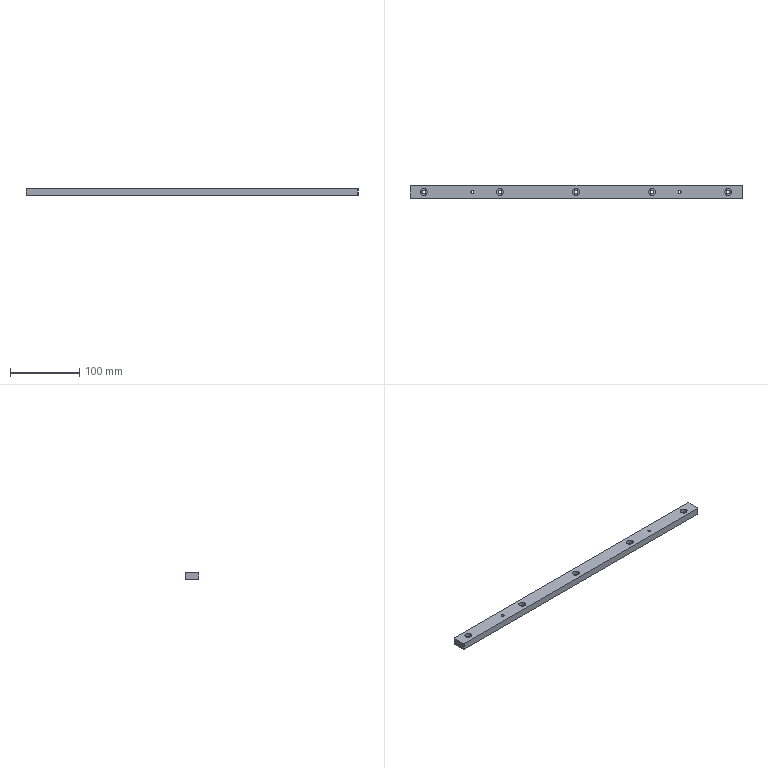Part | SolidWorks | features HoleWzd 2, Chamfer 1, Extrusion 1 | 1 solid | 39 faces | box 480 x 20 x 10 mm | volume 92979 mm3 | cylinder 24 | plane 15 | commonest cylinder face diameters 5.5 x10 10 x10 4 x4
STEP:
#1=CARTESIAN_POINT('',(-152.,0.,0.));
#2=VERTEX_POINT('',#1);
#3=CARTESIAN_POINT('',(-148.,0.,0.));
#4=VERTEX_POINT('',#3);
#5=CARTESIAN_POINT('',(-150.,0.,0.));
#6=DIRECTION('',(0.,0.,1.));
#7=DIRECTION('',(1.,0.,0.));
#8=AXIS2_PLACEMENT_3D('',#5,#6,#7);
#9=CIRCLE('',#8,2.);
#10=EDGE_CURVE('',#2,#4,#9,.T.);
#11=ORIENTED_EDGE('',*,*,#10,.F.);
#12=CARTESIAN_POINT('',(-152.,0.,10.));
#13=VERTEX_POINT('',#12);
#14=CARTESIAN_POINT('',(-152.,0.,10.));
#15=DIRECTION('',(0.,0.,1.));
#16=VECTOR('',#15,1000.);
#17=LINE('',#14,#16);
#18=EDGE_CURVE('',#2,#13,#17,.T.);
#19=ORIENTED_EDGE('',*,*,#18,.T.);
#20=CARTESIAN_POINT('',(-148.,0.,10.));
#21=VERTEX_POINT('',#20);
#22=CARTESIAN_POINT('',(-150.,0.,10.));
#23=DIRECTION('',(0.,0.,1.));
#24=DIRECTION('',(1.,0.,0.));
#25=AXIS2_PLACEMENT_3D('',#22,#23,#24);
#26=CIRCLE('',#25,2.);
#27=EDGE_CURVE('',#13,#21,#26,.T.);
#28=ORIENTED_EDGE('',*,*,#27,.T.);
#29=CARTESIAN_POINT('',(-148.,0.,10.));
#30=DIRECTION('',(0.,0.,1.));
#31=VECTOR('',#30,1000.);
#32=LINE('',#29,#31);
#33=EDGE_CURVE('',#4,#21,#32,.T.);
#34=ORIENTED_EDGE('',*,*,#33,.F.);
#35=EDGE_LOOP('',(#11,#19,#28,#34));
#36=FACE_OUTER_BOUND('',#35,.T.);
#37=CARTESIAN_POINT('',(-150.,0.,10.));
#38=DIRECTION('',(0.,0.,1.));
#39=DIRECTION('',(1.,0.,0.));
#40=AXIS2_PLACEMENT_3D('',#37,#38,#39);
#41=CYLINDRICAL_SURFACE('',#40,2.);
#42=ADVANCED_FACE('',(#36),#41,.F.);
#43=CARTESIAN_POINT('',(148.,0.,0.));
#44=VERTEX_POINT('',#43);
#45=CARTESIAN_POINT('',(152.,0.,0.));
#46=VERTEX_POINT('',#45);
#47=CARTESIAN_POINT('',(150.,0.,0.));
#48=DIRECTION('',(0.,0.,1.));
#49=DIRECTION('',(1.,0.,0.));
#50=AXIS2_PLACEMENT_3D('',#47,#48,#49);
#51=CIRCLE('',#50,2.);
#52=EDGE_CURVE('',#44,#46,#51,.T.);
#53=ORIENTED_EDGE('',*,*,#52,.F.);
#54=CARTESIAN_POINT('',(148.,0.,10.));
#55=VERTEX_POINT('',#54);
#56=CARTESIAN_POINT('',(148.,0.,10.));
#57=DIRECTION('',(0.,0.,1.));
#58=VECTOR('',#57,1000.);
#59=LINE('',#56,#58);
#60=EDGE_CURVE('',#44,#55,#59,.T.);
#61=ORIENTED_EDGE('',*,*,#60,.T.);
#62=CARTESIAN_POINT('',(152.,0.,10.));
#63=VERTEX_POINT('',#62);
#64=CARTESIAN_POINT('',(150.,0.,10.));
#65=DIRECTION('',(0.,0.,1.));
#66=DIRECTION('',(1.,0.,0.));
#67=AXIS2_PLACEMENT_3D('',#64,#65,#66);
#68=CIRCLE('',#67,2.);
#69=EDGE_CURVE('',#55,#63,#68,.T.);
#70=ORIENTED_EDGE('',*,*,#69,.T.);
#71=CARTESIAN_POINT('',(152.,0.,10.));
#72=DIRECTION('',(0.,0.,1.));
#73=VECTOR('',#72,1000.);
#74=LINE('',#71,#73);
#75=EDGE_CURVE('',#46,#63,#74,.T.);
#76=ORIENTED_EDGE('',*,*,#75,.F.);
#77=EDGE_LOOP('',(#53,#61,#70,#76));
#78=FACE_OUTER_BOUND('',#77,.T.);
#79=CARTESIAN_POINT('',(150.,0.,10.));
#80=DIRECTION('',(0.,0.,1.));
#81=DIRECTION('',(1.,0.,0.));
#82=AXIS2_PLACEMENT_3D('',#79,#80,#81);
#83=CYLINDRICAL_SURFACE('',#82,2.);
#84=ADVANCED_FACE('',(#78),#83,.F.);
#85=CARTESIAN_POINT('',(-5.,0.,4.3));
#86=VERTEX_POINT('',#85);
#87=CARTESIAN_POINT('',(5.,0.,4.3));
#88=VERTEX_POINT('',#87);
#89=CARTESIAN_POINT('',(0.,0.,4.3));
#90=DIRECTION('',(0.,0.,1.));
#91=DIRECTION('',(1.,0.,0.));
#92=AXIS2_PLACEMENT_3D('',#89,#90,#91);
#93=CIRCLE('',#92,5.);
#94=EDGE_CURVE('',#86,#88,#93,.T.);
#95=ORIENTED_EDGE('',*,*,#94,.F.);
#96=CARTESIAN_POINT('',(-5.,0.,10.));
#97=VERTEX_POINT('',#96);
#98=CARTESIAN_POINT('',(-5.,0.,10.));
#99=DIRECTION('',(0.,0.,1.));
#100=VECTOR('',#99,1000.);
#101=LINE('',#98,#100);
#102=EDGE_CURVE('',#86,#97,#101,.T.);
#103=ORIENTED_EDGE('',*,*,#102,.T.);
#104=CARTESIAN_POINT('',(5.,0.,10.));
#105=VERTEX_POINT('',#104);
#106=CARTESIAN_POINT('',(0.,0.,10.));
#107=DIRECTION('',(0.,0.,1.));
#108=DIRECTION('',(1.,0.,0.));
#109=AXIS2_PLACEMENT_3D('',#106,#107,#108);
#110=CIRCLE('',#109,5.);
#111=EDGE_CURVE('',#97,#105,#110,.T.);
#112=ORIENTED_EDGE('',*,*,#111,.T.);
#113=CARTESIAN_POINT('',(5.,0.,10.));
#114=DIRECTION('',(0.,0.,1.));
#115=VECTOR('',#114,1000.);
#116=LINE('',#113,#115);
#117=EDGE_CURVE('',#88,#105,#116,.T.);
#118=ORIENTED_EDGE('',*,*,#117,.F.);
#119=EDGE_LOOP('',(#95,#103,#112,#118));
#120=FACE_OUTER_BOUND('',#119,.T.);
#121=CARTESIAN_POINT('',(0.,0.,10.));
#122=DIRECTION('',(0.,0.,1.));
#123=DIRECTION('',(1.,0.,0.));
#124=AXIS2_PLACEMENT_3D('',#121,#122,#123);
#125=CYLINDRICAL_SURFACE('',#124,5.);
#126=ADVANCED_FACE('',(#120),#125,.F.);
#127=CARTESIAN_POINT('',(-2.75,0.,0.));
#128=VERTEX_POINT('',#127);
#129=CARTESIAN_POINT('',(2.75,0.,0.));
#130=VERTEX_POINT('',#129);
#131=CARTESIAN_POINT('',(0.,0.,0.));
#132=DIRECTION('',(0.,0.,1.));
#133=DIRECTION('',(1.,0.,0.));
#134=AXIS2_PLACEMENT_3D('',#131,#132,#133);
#135=CIRCLE('',#134,2.75);
#136=EDGE_CURVE('',#128,#130,#135,.T.);
#137=ORIENTED_EDGE('',*,*,#136,.F.);
#138=CARTESIAN_POINT('',(-2.75,0.,4.3));
#139=VERTEX_POINT('',#138);
#140=CARTESIAN_POINT('',(-2.75,0.,10.));
#141=DIRECTION('',(0.,0.,1.));
#142=VECTOR('',#141,1000.);
#143=LINE('',#140,#142);
#144=EDGE_CURVE('',#128,#139,#143,.T.);
#145=ORIENTED_EDGE('',*,*,#144,.T.);
#146=CARTESIAN_POINT('',(2.75,0.,4.3));
#147=VERTEX_POINT('',#146);
#148=CARTESIAN_POINT('',(0.,0.,4.3));
#149=DIRECTION('',(0.,0.,1.));
#150=DIRECTION('',(1.,0.,0.));
#151=AXIS2_PLACEMENT_3D('',#148,#149,#150);
#152=CIRCLE('',#151,2.75);
#153=EDGE_CURVE('',#139,#147,#152,.T.);
#154=ORIENTED_EDGE('',*,*,#153,.T.);
#155=CARTESIAN_POINT('',(2.75,0.,10.));
#156=DIRECTION('',(0.,0.,1.));
#157=VECTOR('',#156,1000.);
#158=LINE('',#155,#157);
#159=EDGE_CURVE('',#130,#147,#158,.T.);
#160=ORIENTED_EDGE('',*,*,#159,.F.);
#161=EDGE_LOOP('',(#137,#145,#154,#160));
#162=FACE_OUTER_BOUND('',#161,.T.);
#163=CARTESIAN_POINT('',(0.,0.,10.));
#164=DIRECTION('',(0.,0.,1.));
#165=DIRECTION('',(1.,0.,0.));
#166=AXIS2_PLACEMENT_3D('',#163,#164,#165);
#167=CYLINDRICAL_SURFACE('',#166,2.75);
#168=ADVANCED_FACE('',(#162),#167,.F.);
#169=CARTESIAN_POINT('',(-115.,0.,4.3));
#170=VERTEX_POINT('',#169);
#171=CARTESIAN_POINT('',(-105.,0.,4.3));
#172=VERTEX_POINT('',#171);
#173=CARTESIAN_POINT('',(-110.,0.,4.3));
#174=DIRECTION('',(0.,0.,1.));
#175=DIRECTION('',(1.,0.,0.));
#176=AXIS2_PLACEMENT_3D('',#173,#174,#175);
#177=CIRCLE('',#176,5.);
#178=EDGE_CURVE('',#170,#172,#177,.T.);
#179=ORIENTED_EDGE('',*,*,#178,.F.);
#180=CARTESIAN_POINT('',(-115.,0.,10.));
#181=VERTEX_POINT('',#180);
#182=CARTESIAN_POINT('',(-115.,0.,10.));
#183=DIRECTION('',(0.,0.,1.));
#184=VECTOR('',#183,1000.);
#185=LINE('',#182,#184);
#186=EDGE_CURVE('',#170,#181,#185,.T.);
#187=ORIENTED_EDGE('',*,*,#186,.T.);
#188=CARTESIAN_POINT('',(-105.,0.,10.));
#189=VERTEX_POINT('',#188);
#190=CARTESIAN_POINT('',(-110.,0.,10.));
#191=DIRECTION('',(0.,0.,1.));
#192=DIRECTION('',(1.,0.,0.));
#193=AXIS2_PLACEMENT_3D('',#190,#191,#192);
#194=CIRCLE('',#193,5.);
#195=EDGE_CURVE('',#181,#189,#194,.T.);
#196=ORIENTED_EDGE('',*,*,#195,.T.);
#197=CARTESIAN_POINT('',(-105.,0.,10.));
#198=DIRECTION('',(0.,0.,1.));
#199=VECTOR('',#198,1000.);
#200=LINE('',#197,#199);
#201=EDGE_CURVE('',#172,#189,#200,.T.);
#202=ORIENTED_EDGE('',*,*,#201,.F.);
#203=EDGE_LOOP('',(#179,#187,#196,#202));
#204=FACE_OUTER_BOUND('',#203,.T.);
#205=CARTESIAN_POINT('',(-110.,0.,10.));
#206=DIRECTION('',(0.,0.,1.));
#207=DIRECTION('',(1.,0.,0.));
#208=AXIS2_PLACEMENT_3D('',#205,#206,#207);
#209=CYLINDRICAL_SURFACE('',#208,5.);
#210=ADVANCED_FACE('',(#204),#209,.F.);
#211=CARTESIAN_POINT('',(-112.75,0.,0.));
#212=VERTEX_POINT('',#211);
#213=CARTESIAN_POINT('',(-107.25,0.,0.));
#214=VERTEX_POINT('',#213);
#215=CARTESIAN_POINT('',(-110.,0.,0.));
#216=DIRECTION('',(0.,0.,1.));
#217=DIRECTION('',(1.,0.,0.));
#218=AXIS2_PLACEMENT_3D('',#215,#216,#217);
#219=CIRCLE('',#218,2.75);
#220=EDGE_CURVE('',#212,#214,#219,.T.);
#221=ORIENTED_EDGE('',*,*,#220,.F.);
#222=CARTESIAN_POINT('',(-112.75,0.,4.3));
#223=VERTEX_POINT('',#222);
#224=CARTESIAN_POINT('',(-112.75,0.,10.));
#225=DIRECTION('',(0.,0.,1.));
#226=VECTOR('',#225,1000.);
#227=LINE('',#224,#226);
#228=EDGE_CURVE('',#212,#223,#227,.T.);
#229=ORIENTED_EDGE('',*,*,#228,.T.);
#230=CARTESIAN_POINT('',(-107.25,0.,4.3));
#231=VERTEX_POINT('',#230);
#232=CARTESIAN_POINT('',(-110.,0.,4.3));
#233=DIRECTION('',(0.,0.,1.));
#234=DIRECTION('',(1.,0.,0.));
#235=AXIS2_PLACEMENT_3D('',#232,#233,#234);
#236=CIRCLE('',#235,2.75);
#237=EDGE_CURVE('',#223,#231,#236,.T.);
#238=ORIENTED_EDGE('',*,*,#237,.T.);
#239=CARTESIAN_POINT('',(-107.25,0.,10.));
#240=DIRECTION('',(0.,0.,1.));
#241=VECTOR('',#240,1000.);
#242=LINE('',#239,#241);
#243=EDGE_CURVE('',#214,#231,#242,.T.);
#244=ORIENTED_EDGE('',*,*,#243,.F.);
#245=EDGE_LOOP('',(#221,#229,#238,#244));
#246=FACE_OUTER_BOUND('',#245,.T.);
#247=CARTESIAN_POINT('',(-110.,0.,10.));
#248=DIRECTION('',(0.,0.,1.));
#249=DIRECTION('',(1.,0.,0.));
#250=AXIS2_PLACEMENT_3D('',#247,#248,#249);
#251=CYLINDRICAL_SURFACE('',#250,2.75);
#252=ADVANCED_FACE('',(#246),#251,.F.);
#253=CARTESIAN_POINT('',(105.,0.,4.3));
#254=VERTEX_POINT('',#253);
#255=CARTESIAN_POINT('',(115.,0.,4.3));
#256=VERTEX_POINT('',#255);
#257=CARTESIAN_POINT('',(110.,0.,4.3));
#258=DIRECTION('',(0.,0.,1.));
#259=DIRECTION('',(1.,0.,0.));
#260=AXIS2_PLACEMENT_3D('',#257,#258,#259);
#261=CIRCLE('',#260,5.);
#262=EDGE_CURVE('',#254,#256,#261,.T.);
#263=ORIENTED_EDGE('',*,*,#262,.F.);
#264=CARTESIAN_POINT('',(105.,0.,10.));
#265=VERTEX_POINT('',#264);
#266=CARTESIAN_POINT('',(105.,0.,10.));
#267=DIRECTION('',(0.,0.,1.));
#268=VECTOR('',#267,1000.);
#269=LINE('',#266,#268);
#270=EDGE_CURVE('',#254,#265,#269,.T.);
#271=ORIENTED_EDGE('',*,*,#270,.T.);
#272=CARTESIAN_POINT('',(115.,0.,10.));
#273=VERTEX_POINT('',#272);
#274=CARTESIAN_POINT('',(110.,0.,10.));
#275=DIRECTION('',(0.,0.,1.));
#276=DIRECTION('',(1.,0.,0.));
#277=AXIS2_PLACEMENT_3D('',#274,#275,#276);
#278=CIRCLE('',#277,5.);
#279=EDGE_CURVE('',#265,#273,#278,.T.);
#280=ORIENTED_EDGE('',*,*,#279,.T.);
#281=CARTESIAN_POINT('',(115.,0.,10.));
#282=DIRECTION('',(0.,0.,1.));
#283=VECTOR('',#282,1000.);
#284=LINE('',#281,#283);
#285=EDGE_CURVE('',#256,#273,#284,.T.);
#286=ORIENTED_EDGE('',*,*,#285,.F.);
#287=EDGE_LOOP('',(#263,#271,#280,#286));
#288=FACE_OUTER_BOUND('',#287,.T.);
#289=CARTESIAN_POINT('',(110.,0.,10.));
#290=DIRECTION('',(0.,0.,1.));
#291=DIRECTION('',(1.,0.,0.));
#292=AXIS2_PLACEMENT_3D('',#289,#290,#291);
#293=CYLINDRICAL_SURFACE('',#292,5.);
#294=ADVANCED_FACE('',(#288),#293,.F.);
#295=CARTESIAN_POINT('',(107.25,0.,0.));
#296=VERTEX_POINT('',#295);
#297=CARTESIAN_POINT('',(112.75,0.,0.));
#298=VERTEX_POINT('',#297);
#299=CARTESIAN_POINT('',(110.,0.,0.));
#300=DIRECTION('',(0.,0.,1.));
#301=DIRECTION('',(1.,0.,0.));
#302=AXIS2_PLACEMENT_3D('',#299,#300,#301);
#303=CIRCLE('',#302,2.75);
#304=EDGE_CURVE('',#296,#298,#303,.T.);
#305=ORIENTED_EDGE('',*,*,#304,.F.);
#306=CARTESIAN_POINT('',(107.25,0.,4.3));
#307=VERTEX_POINT('',#306);
#308=CARTESIAN_POINT('',(107.25,0.,10.));
#309=DIRECTION('',(0.,0.,1.));
#310=VECTOR('',#309,1000.);
#311=LINE('',#308,#310);
#312=EDGE_CURVE('',#296,#307,#311,.T.);
#313=ORIENTED_EDGE('',*,*,#312,.T.);
#314=CARTESIAN_POINT('',(112.75,0.,4.3));
#315=VERTEX_POINT('',#314);
#316=CARTESIAN_POINT('',(110.,0.,4.3));
#317=DIRECTION('',(0.,0.,1.));
#318=DIRECTION('',(1.,0.,0.));
#319=AXIS2_PLACEMENT_3D('',#316,#317,#318);
#320=CIRCLE('',#319,2.75);
#321=EDGE_CURVE('',#307,#315,#320,.T.);
#322=ORIENTED_EDGE('',*,*,#321,.T.);
#323=CARTESIAN_POINT('',(112.75,0.,10.));
#324=DIRECTION('',(0.,0.,1.));
#325=VECTOR('',#324,1000.);
#326=LINE('',#323,#325);
#327=EDGE_CURVE('',#298,#315,#326,.T.);
#328=ORIENTED_EDGE('',*,*,#327,.F.);
#329=EDGE_LOOP('',(#305,#313,#322,#328));
#330=FACE_OUTER_BOUND('',#329,.T.);
#331=CARTESIAN_POINT('',(110.,0.,10.));
#332=DIRECTION('',(0.,0.,1.));
#333=DIRECTION('',(1.,0.,0.));
#334=AXIS2_PLACEMENT_3D('',#331,#332,#333);
#335=CYLINDRICAL_SURFACE('',#334,2.75);
#336=ADVANCED_FACE('',(#330),#335,.F.);
#337=CARTESIAN_POINT('',(215.,0.,4.3));
#338=VERTEX_POINT('',#337);
#339=CARTESIAN_POINT('',(225.,0.,4.3));
#340=VERTEX_POINT('',#339);
#341=CARTESIAN_POINT('',(220.,0.,4.3));
#342=DIRECTION('',(0.,0.,1.));
#343=DIRECTION('',(1.,0.,0.));
#344=AXIS2_PLACEMENT_3D('',#341,#342,#343);
#345=CIRCLE('',#344,5.);
#346=EDGE_CURVE('',#338,#340,#345,.T.);
#347=ORIENTED_EDGE('',*,*,#346,.F.);
#348=CARTESIAN_POINT('',(215.,0.,10.));
#349=VERTEX_POINT('',#348);
#350=CARTESIAN_POINT('',(215.,0.,10.));
#351=DIRECTION('',(0.,0.,1.));
#352=VECTOR('',#351,1000.);
#353=LINE('',#350,#352);
#354=EDGE_CURVE('',#338,#349,#353,.T.);
#355=ORIENTED_EDGE('',*,*,#354,.T.);
#356=CARTESIAN_POINT('',(225.,0.,10.));
#357=VERTEX_POINT('',#356);
#358=CARTESIAN_POINT('',(220.,0.,10.));
#359=DIRECTION('',(0.,0.,1.));
#360=DIRECTION('',(1.,0.,0.));
#361=AXIS2_PLACEMENT_3D('',#358,#359,#360);
#362=CIRCLE('',#361,5.);
#363=EDGE_CURVE('',#349,#357,#362,.T.);
#364=ORIENTED_EDGE('',*,*,#363,.T.);
#365=CARTESIAN_POINT('',(225.,0.,10.));
#366=DIRECTION('',(0.,0.,1.));
#367=VECTOR('',#366,1000.);
#368=LINE('',#365,#367);
#369=EDGE_CURVE('',#340,#357,#368,.T.);
#370=ORIENTED_EDGE('',*,*,#369,.F.);
#371=EDGE_LOOP('',(#347,#355,#364,#370));
#372=FACE_OUTER_BOUND('',#371,.T.);
#373=CARTESIAN_POINT('',(220.,0.,10.));
#374=DIRECTION('',(0.,0.,1.));
#375=DIRECTION('',(1.,0.,0.));
#376=AXIS2_PLACEMENT_3D('',#373,#374,#375);
#377=CYLINDRICAL_SURFACE('',#376,5.);
#378=ADVANCED_FACE('',(#372),#377,.F.);
#379=CARTESIAN_POINT('',(217.25,0.,0.));
#380=VERTEX_POINT('',#379);
#381=CARTESIAN_POINT('',(222.75,0.,0.));
#382=VERTEX_POINT('',#381);
#383=CARTESIAN_POINT('',(220.,0.,0.));
#384=DIRECTION('',(0.,0.,1.));
#385=DIRECTION('',(1.,0.,0.));
#386=AXIS2_PLACEMENT_3D('',#383,#384,#385);
#387=CIRCLE('',#386,2.75);
#388=EDGE_CURVE('',#380,#382,#387,.T.);
#389=ORIENTED_EDGE('',*,*,#388,.F.);
#390=CARTESIAN_POINT('',(217.25,0.,4.3));
#391=VERTEX_POINT('',#390);
#392=CARTESIAN_POINT('',(217.25,0.,10.));
#393=DIRECTION('',(0.,0.,1.));
#394=VECTOR('',#393,1000.);
#395=LINE('',#392,#394);
#396=EDGE_CURVE('',#380,#391,#395,.T.);
#397=ORIENTED_EDGE('',*,*,#396,.T.);
#398=CARTESIAN_POINT('',(222.75,0.,4.3));
#399=VERTEX_POINT('',#398);
#400=CARTESIAN_POINT('',(220.,0.,4.3));
#401=DIRECTION('',(0.,0.,1.));
#402=DIRECTION('',(1.,0.,0.));
#403=AXIS2_PLACEMENT_3D('',#400,#401,#402);
#404=CIRCLE('',#403,2.75);
#405=EDGE_CURVE('',#391,#399,#404,.T.);
#406=ORIENTED_EDGE('',*,*,#405,.T.);
#407=CARTESIAN_POINT('',(222.75,0.,10.));
#408=DIRECTION('',(0.,0.,1.));
#409=VECTOR('',#408,1000.);
#410=LINE('',#407,#409);
#411=EDGE_CURVE('',#382,#399,#410,.T.);
#412=ORIENTED_EDGE('',*,*,#411,.F.);
#413=EDGE_LOOP('',(#389,#397,#406,#412));
#414=FACE_OUTER_BOUND('',#413,.T.);
#415=CARTESIAN_POINT('',(220.,0.,10.));
#416=DIRECTION('',(0.,0.,1.));
#417=DIRECTION('',(1.,0.,0.));
#418=AXIS2_PLACEMENT_3D('',#415,#416,#417);
#419=CYLINDRICAL_SURFACE('',#418,2.75);
#420=ADVANCED_FACE('',(#414),#419,.F.);
#421=CARTESIAN_POINT('',(-225.,0.,4.3));
#422=VERTEX_POINT('',#421);
#423=CARTESIAN_POINT('',(-215.,0.,4.3));
#424=VERTEX_POINT('',#423);
#425=CARTESIAN_POINT('',(-220.,0.,4.3));
#426=DIRECTION('',(0.,0.,1.));
#427=DIRECTION('',(1.,0.,0.));
#428=AXIS2_PLACEMENT_3D('',#425,#426,#427);
#429=CIRCLE('',#428,5.);
#430=EDGE_CURVE('',#422,#424,#429,.T.);
#431=ORIENTED_EDGE('',*,*,#430,.F.);
#432=CARTESIAN_POINT('',(-225.,0.,10.));
#433=VERTEX_POINT('',#432);
#434=CARTESIAN_POINT('',(-225.,0.,10.));
#435=DIRECTION('',(0.,0.,1.));
#436=VECTOR('',#435,1000.);
#437=LINE('',#434,#436);
#438=EDGE_CURVE('',#422,#433,#437,.T.);
#439=ORIENTED_EDGE('',*,*,#438,.T.);
#440=CARTESIAN_POINT('',(-215.,0.,10.));
#441=VERTEX_POINT('',#440);
#442=CARTESIAN_POINT('',(-220.,0.,10.));
#443=DIRECTION('',(0.,0.,1.));
#444=DIRECTION('',(1.,0.,0.));
#445=AXIS2_PLACEMENT_3D('',#442,#443,#444);
#446=CIRCLE('',#445,5.);
#447=EDGE_CURVE('',#433,#441,#446,.T.);
#448=ORIENTED_EDGE('',*,*,#447,.T.);
#449=CARTESIAN_POINT('',(-215.,0.,10.));
#450=DIRECTION('',(0.,0.,1.));
#451=VECTOR('',#450,1000.);
#452=LINE('',#449,#451);
#453=EDGE_CURVE('',#424,#441,#452,.T.);
#454=ORIENTED_EDGE('',*,*,#453,.F.);
#455=EDGE_LOOP('',(#431,#439,#448,#454));
#456=FACE_OUTER_BOUND('',#455,.T.);
#457=CARTESIAN_POINT('',(-220.,0.,10.));
#458=DIRECTION('',(0.,0.,1.));
#459=DIRECTION('',(1.,0.,0.));
#460=AXIS2_PLACEMENT_3D('',#457,#458,#459);
#461=CYLINDRICAL_SURFACE('',#460,5.);
#462=ADVANCED_FACE('',(#456),#461,.F.);
#463=CARTESIAN_POINT('',(-222.75,0.,0.));
#464=VERTEX_POINT('',#463);
#465=CARTESIAN_POINT('',(-217.25,0.,0.));
#466=VERTEX_POINT('',#465);
#467=CARTESIAN_POINT('',(-220.,0.,0.));
#468=DIRECTION('',(0.,0.,1.));
#469=DIRECTION('',(1.,0.,0.));
#470=AXIS2_PLACEMENT_3D('',#467,#468,#469);
#471=CIRCLE('',#470,2.75);
#472=EDGE_CURVE('',#464,#466,#471,.T.);
#473=ORIENTED_EDGE('',*,*,#472,.F.);
#474=CARTESIAN_POINT('',(-222.75,0.,4.3));
#475=VERTEX_POINT('',#474);
#476=CARTESIAN_POINT('',(-222.75,0.,10.));
#477=DIRECTION('',(0.,0.,1.));
#478=VECTOR('',#477,1000.);
#479=LINE('',#476,#478);
#480=EDGE_CURVE('',#464,#475,#479,.T.);
#481=ORIENTED_EDGE('',*,*,#480,.T.);
#482=CARTESIAN_POINT('',(-217.25,0.,4.3));
#483=VERTEX_POINT('',#482);
#484=CARTESIAN_POINT('',(-220.,0.,4.3));
#485=DIRECTION('',(0.,0.,1.));
#486=DIRECTION('',(1.,0.,0.));
#487=AXIS2_PLACEMENT_3D('',#484,#485,#486);
#488=CIRCLE('',#487,2.75);
#489=EDGE_CURVE('',#475,#483,#488,.T.);
#490=ORIENTED_EDGE('',*,*,#489,.T.);
#491=CARTESIAN_POINT('',(-217.25,0.,10.));
#492=DIRECTION('',(0.,0.,1.));
#493=VECTOR('',#492,1000.);
#494=LINE('',#491,#493);
#495=EDGE_CURVE('',#466,#483,#494,.T.);
#496=ORIENTED_EDGE('',*,*,#495,.F.);
#497=EDGE_LOOP('',(#473,#481,#490,#496));
#498=FACE_OUTER_BOUND('',#497,.T.);
#499=CARTESIAN_POINT('',(-220.,0.,10.));
#500=DIRECTION('',(0.,0.,1.));
#501=DIRECTION('',(1.,0.,0.));
#502=AXIS2_PLACEMENT_3D('',#499,#500,#501);
#503=CYLINDRICAL_SURFACE('',#502,2.75);
#504=ADVANCED_FACE('',(#498),#503,.F.);
#505=CARTESIAN_POINT('',(240.,-9.,10.));
#506=VERTEX_POINT('',#505);
#507=CARTESIAN_POINT('',(240.,9.,10.));
#508=VERTEX_POINT('',#507);
#509=CARTESIAN_POINT('',(240.,10.,10.));
#510=DIRECTION('',(0.,1.,0.));
#511=VECTOR('',#510,1000.);
#512=LINE('',#509,#511);
#513=EDGE_CURVE('',#506,#508,#512,.T.);
#514=ORIENTED_EDGE('',*,*,#513,.F.);
#515=CARTESIAN_POINT('',(240.,-9.,0.));
#516=VERTEX_POINT('',#515);
#517=CARTESIAN_POINT('',(240.,-9.,10.));
#518=DIRECTION('',(0.,0.,-1.));
#519=VECTOR('',#518,1000.);
#520=LINE('',#517,#519);
#521=EDGE_CURVE('',#506,#516,#520,.T.);
#522=ORIENTED_EDGE('',*,*,#521,.T.);
#523=CARTESIAN_POINT('',(240.,9.,0.));
#524=VERTEX_POINT('',#523);
#525=CARTESIAN_POINT('',(240.,10.,0.));
#526=DIRECTION('',(0.,1.,0.));
#527=VECTOR('',#526,1000.);
#528=LINE('',#525,#527);
#529=EDGE_CURVE('',#516,#524,#528,.T.);
#530=ORIENTED_EDGE('',*,*,#529,.T.);
#531=CARTESIAN_POINT('',(240.,9.,10.));
#532=DIRECTION('',(0.,0.,1.));
#533=VECTOR('',#532,1000.);
#534=LINE('',#531,#533);
#535=EDGE_CURVE('',#524,#508,#534,.T.);
#536=ORIENTED_EDGE('',*,*,#535,.T.);
#537=EDGE_LOOP('',(#514,#522,#530,#536));
#538=FACE_OUTER_BOUND('',#537,.T.);
#539=CARTESIAN_POINT('',(240.,10.,10.));
#540=DIRECTION('',(-1.,0.,0.));
#541=DIRECTION('',(0.,0.,1.));
#542=AXIS2_PLACEMENT_3D('',#539,#540,#541);
#543=PLANE('',#542);
#544=ADVANCED_FACE('',(#538),#543,.F.);
#545=CARTESIAN_POINT('',(239.,10.,10.));
#546=VERTEX_POINT('',#545);
#547=CARTESIAN_POINT('',(-239.,10.,10.));
#548=VERTEX_POINT('',#547);
#549=CARTESIAN_POINT('',(-240.,10.,10.));
#550=DIRECTION('',(-1.,0.,0.));
#551=VECTOR('',#550,1000.);
#552=LINE('',#549,#551);
#553=EDGE_CURVE('',#546,#548,#552,.T.);
#554=ORIENTED_EDGE('',*,*,#553,.F.);
#555=CARTESIAN_POINT('',(239.,10.,0.));
#556=VERTEX_POINT('',#555);
#557=CARTESIAN_POINT('',(239.,10.,10.));
#558=DIRECTION('',(0.,0.,-1.));
#559=VECTOR('',#558,1000.);
#560=LINE('',#557,#559);
#561=EDGE_CURVE('',#546,#556,#560,.T.);
#562=ORIENTED_EDGE('',*,*,#561,.T.);
#563=CARTESIAN_POINT('',(-239.,10.,0.));
#564=VERTEX_POINT('',#563);
#565=CARTESIAN_POINT('',(-240.,10.,0.));
#566=DIRECTION('',(-1.,0.,0.));
#567=VECTOR('',#566,1000.);
#568=LINE('',#565,#567);
#569=EDGE_CURVE('',#556,#564,#568,.T.);
#570=ORIENTED_EDGE('',*,*,#569,.T.);
#571=CARTESIAN_POINT('',(-239.,10.,10.));
#572=DIRECTION('',(0.,0.,1.));
#573=VECTOR('',#572,1000.);
#574=LINE('',#571,#573);
#575=EDGE_CURVE('',#564,#548,#574,.T.);
#576=ORIENTED_EDGE('',*,*,#575,.T.);
#577=EDGE_LOOP('',(#554,#562,#570,#576));
#578=FACE_OUTER_BOUND('',#577,.T.);
#579=CARTESIAN_POINT('',(-240.,10.,10.));
#580=DIRECTION('',(0.,-1.,0.));
#581=DIRECTION('',(0.,0.,-1.));
#582=AXIS2_PLACEMENT_3D('',#579,#580,#581);
#583=PLANE('',#582);
#584=ADVANCED_FACE('',(#578),#583,.F.);
#585=CARTESIAN_POINT('',(-240.,9.,10.));
#586=VERTEX_POINT('',#585);
#587=CARTESIAN_POINT('',(-240.,-9.,10.));
#588=VERTEX_POINT('',#587);
#589=CARTESIAN_POINT('',(-240.,10.,10.));
#590=DIRECTION('',(0.,-1.,0.));
#591=VECTOR('',#590,1000.);
#592=LINE('',#589,#591);
#593=EDGE_CURVE('',#586,#588,#592,.T.);
#594=ORIENTED_EDGE('',*,*,#593,.F.);
#595=CARTESIAN_POINT('',(-240.,9.,0.));
#596=VERTEX_POINT('',#595);
#597=CARTESIAN_POINT('',(-240.,9.,10.));
#598=DIRECTION('',(0.,0.,-1.));
#599=VECTOR('',#598,1000.);
#600=LINE('',#597,#599);
#601=EDGE_CURVE('',#586,#596,#600,.T.);
#602=ORIENTED_EDGE('',*,*,#601,.T.);
#603=CARTESIAN_POINT('',(-240.,-9.,0.));
#604=VERTEX_POINT('',#603);
#605=CARTESIAN_POINT('',(-240.,10.,0.));
#606=DIRECTION('',(0.,-1.,0.));
#607=VECTOR('',#606,1000.);
#608=LINE('',#605,#607);
#609=EDGE_CURVE('',#596,#604,#608,.T.);
#610=ORIENTED_EDGE('',*,*,#609,.T.);
#611=CARTESIAN_POINT('',(-240.,-9.,10.));
#612=DIRECTION('',(0.,0.,1.));
#613=VECTOR('',#612,1000.);
#614=LINE('',#611,#613);
#615=EDGE_CURVE('',#604,#588,#614,.T.);
#616=ORIENTED_EDGE('',*,*,#615,.T.);
#617=EDGE_LOOP('',(#594,#602,#610,#616));
#618=FACE_OUTER_BOUND('',#617,.T.);
#619=CARTESIAN_POINT('',(-240.,10.,10.));
#620=DIRECTION('',(1.,0.,0.));
#621=DIRECTION('',(0.,0.,-1.));
#622=AXIS2_PLACEMENT_3D('',#619,#620,#621);
#623=PLANE('',#622);
#624=ADVANCED_FACE('',(#618),#623,.F.);
#625=CARTESIAN_POINT('',(-239.,-10.,0.));
#626=VERTEX_POINT('',#625);
#627=CARTESIAN_POINT('',(239.,-10.,0.));
#628=VERTEX_POINT('',#627);
#629=CARTESIAN_POINT('',(-240.,-10.,0.));
#630=DIRECTION('',(1.,0.,0.));
#631=VECTOR('',#630,1000.);
#632=LINE('',#629,#631);
#633=EDGE_CURVE('',#626,#628,#632,.T.);
#634=ORIENTED_EDGE('',*,*,#633,.T.);
#635=CARTESIAN_POINT('',(239.,-10.,10.));
#636=VERTEX_POINT('',#635);
#637=CARTESIAN_POINT('',(239.,-10.,10.));
#638=DIRECTION('',(0.,0.,1.));
#639=VECTOR('',#638,1000.);
#640=LINE('',#637,#639);
#641=EDGE_CURVE('',#628,#636,#640,.T.);
#642=ORIENTED_EDGE('',*,*,#641,.T.);
#643=CARTESIAN_POINT('',(-239.,-10.,10.));
#644=VERTEX_POINT('',#643);
#645=CARTESIAN_POINT('',(-240.,-10.,10.));
#646=DIRECTION('',(1.,0.,0.));
#647=VECTOR('',#646,1000.);
#648=LINE('',#645,#647);
#649=EDGE_CURVE('',#644,#636,#648,.T.);
#650=ORIENTED_EDGE('',*,*,#649,.F.);
#651=CARTESIAN_POINT('',(-239.,-10.,10.));
#652=DIRECTION('',(0.,0.,-1.));
#653=VECTOR('',#652,1000.);
#654=LINE('',#651,#653);
#655=EDGE_CURVE('',#644,#626,#654,.T.);
#656=ORIENTED_EDGE('',*,*,#655,.T.);
#657=EDGE_LOOP('',(#634,#642,#650,#656));
#658=FACE_OUTER_BOUND('',#657,.T.);
#659=CARTESIAN_POINT('',(-240.,-10.,10.));
#660=DIRECTION('',(0.,1.,0.));
#661=DIRECTION('',(0.,0.,1.));
#662=AXIS2_PLACEMENT_3D('',#659,#660,#661);
#663=PLANE('',#662);
#664=ADVANCED_FACE('',(#658),#663,.F.);
#665=CARTESIAN_POINT('',(-150.,0.,10.));
#666=DIRECTION('',(0.,0.,1.));
#667=DIRECTION('',(1.,0.,0.));
#668=AXIS2_PLACEMENT_3D('',#665,#666,#667);
#669=CIRCLE('',#668,2.);
#670=EDGE_CURVE('',#21,#13,#669,.T.);
#671=ORIENTED_EDGE('',*,*,#670,.F.);
#672=ORIENTED_EDGE('',*,*,#27,.F.);
#673=EDGE_LOOP('',(#671,#672));
#674=FACE_BOUND('',#673,.T.);
#675=CARTESIAN_POINT('',(150.,0.,10.));
#676=DIRECTION('',(0.,0.,1.));
#677=DIRECTION('',(1.,0.,0.));
#678=AXIS2_PLACEMENT_3D('',#675,#676,#677);
#679=CIRCLE('',#678,2.);
#680=EDGE_CURVE('',#63,#55,#679,.T.);
#681=ORIENTED_EDGE('',*,*,#680,.F.);
#682=ORIENTED_EDGE('',*,*,#69,.F.);
#683=EDGE_LOOP('',(#681,#682));
#684=FACE_BOUND('',#683,.T.);
#685=CARTESIAN_POINT('',(0.,0.,10.));
#686=DIRECTION('',(0.,0.,1.));
#687=DIRECTION('',(1.,0.,0.));
#688=AXIS2_PLACEMENT_3D('',#685,#686,#687);
#689=CIRCLE('',#688,5.);
#690=EDGE_CURVE('',#105,#97,#689,.T.);
#691=ORIENTED_EDGE('',*,*,#690,.F.);
#692=ORIENTED_EDGE('',*,*,#111,.F.);
#693=EDGE_LOOP('',(#691,#692));
#694=FACE_BOUND('',#693,.T.);
#695=CARTESIAN_POINT('',(-110.,0.,10.));
#696=DIRECTION('',(0.,0.,1.));
#697=DIRECTION('',(1.,0.,0.));
#698=AXIS2_PLACEMENT_3D('',#695,#696,#697);
#699=CIRCLE('',#698,5.);
#700=EDGE_CURVE('',#189,#181,#699,.T.);
#701=ORIENTED_EDGE('',*,*,#700,.F.);
#702=ORIENTED_EDGE('',*,*,#195,.F.);
#703=EDGE_LOOP('',(#701,#702));
#704=FACE_BOUND('',#703,.T.);
#705=CARTESIAN_POINT('',(110.,0.,10.));
#706=DIRECTION('',(0.,0.,1.));
#707=DIRECTION('',(1.,0.,0.));
#708=AXIS2_PLACEMENT_3D('',#705,#706,#707);
#709=CIRCLE('',#708,5.);
#710=EDGE_CURVE('',#273,#265,#709,.T.);
#711=ORIENTED_EDGE('',*,*,#710,.F.);
#712=ORIENTED_EDGE('',*,*,#279,.F.);
#713=EDGE_LOOP('',(#711,#712));
#714=FACE_BOUND('',#713,.T.);
#715=CARTESIAN_POINT('',(220.,0.,10.));
#716=DIRECTION('',(0.,0.,1.));
#717=DIRECTION('',(1.,0.,0.));
#718=AXIS2_PLACEMENT_3D('',#715,#716,#717);
#719=CIRCLE('',#718,5.);
#720=EDGE_CURVE('',#357,#349,#719,.T.);
#721=ORIENTED_EDGE('',*,*,#720,.F.);
#722=ORIENTED_EDGE('',*,*,#363,.F.);
#723=EDGE_LOOP('',(#721,#722));
#724=FACE_BOUND('',#723,.T.);
#725=CARTESIAN_POINT('',(-220.,0.,10.));
#726=DIRECTION('',(0.,0.,1.));
#727=DIRECTION('',(1.,0.,0.));
#728=AXIS2_PLACEMENT_3D('',#725,#726,#727);
#729=CIRCLE('',#728,5.);
#730=EDGE_CURVE('',#441,#433,#729,.T.);
#731=ORIENTED_EDGE('',*,*,#730,.F.);
#732=ORIENTED_EDGE('',*,*,#447,.F.);
#733=EDGE_LOOP('',(#731,#732));
#734=FACE_BOUND('',#733,.T.);
#735=ORIENTED_EDGE('',*,*,#649,.T.);
#736=CARTESIAN_POINT('',(239.5,-9.5,10.));
#737=DIRECTION('',(0.7071,0.7071,0.));
#738=VECTOR('',#737,1000.);
#739=LINE('',#736,#738);
#740=EDGE_CURVE('',#636,#506,#739,.T.);
#741=ORIENTED_EDGE('',*,*,#740,.T.);
#742=ORIENTED_EDGE('',*,*,#513,.T.);
#743=CARTESIAN_POINT('',(249.5,-0.5,10.));
#744=DIRECTION('',(-0.7071,0.7071,0.));
#745=VECTOR('',#744,1000.);
#746=LINE('',#743,#745);
#747=EDGE_CURVE('',#508,#546,#746,.T.);
#748=ORIENTED_EDGE('',*,*,#747,.T.);
#749=ORIENTED_EDGE('',*,*,#553,.T.);
#750=CARTESIAN_POINT('',(-9.5,239.5,10.));
#751=DIRECTION('',(-0.7071,-0.7071,0.));
#752=VECTOR('',#751,1000.);
#753=LINE('',#750,#752);
#754=EDGE_CURVE('',#548,#586,#753,.T.);
#755=ORIENTED_EDGE('',*,*,#754,.T.);
#756=ORIENTED_EDGE('',*,*,#593,.T.);
#757=CARTESIAN_POINT('',(0.5,-249.5,10.));
#758=DIRECTION('',(0.7071,-0.7071,0.));
#759=VECTOR('',#758,1000.);
#760=LINE('',#757,#759);
#761=EDGE_CURVE('',#588,#644,#760,.T.);
#762=ORIENTED_EDGE('',*,*,#761,.T.);
#763=EDGE_LOOP('',(#735,#741,#742,#748,#749,#755,#756,#762));
#764=FACE_OUTER_BOUND('',#763,.T.);
#765=CARTESIAN_POINT('',(240.,-10.,10.));
#766=DIRECTION('',(0.,0.,1.));
#767=DIRECTION('',(1.,0.,0.));
#768=AXIS2_PLACEMENT_3D('',#765,#766,#767);
#769=PLANE('',#768);
#770=ADVANCED_FACE('',(#674,#684,#694,#704,#714,#724,#734,#764),#769,.T.);
#771=CARTESIAN_POINT('',(-150.,0.,0.));
#772=DIRECTION('',(0.,0.,1.));
#773=DIRECTION('',(1.,0.,0.));
#774=AXIS2_PLACEMENT_3D('',#771,#772,#773);
#775=CIRCLE('',#774,2.);
#776=EDGE_CURVE('',#4,#2,#775,.T.);
#777=ORIENTED_EDGE('',*,*,#776,.T.);
#778=ORIENTED_EDGE('',*,*,#10,.T.);
#779=EDGE_LOOP('',(#777,#778));
#780=FACE_BOUND('',#779,.T.);
#781=CARTESIAN_POINT('',(150.,0.,0.));
#782=DIRECTION('',(0.,0.,1.));
#783=DIRECTION('',(1.,0.,0.));
#784=AXIS2_PLACEMENT_3D('',#781,#782,#783);
#785=CIRCLE('',#784,2.);
#786=EDGE_CURVE('',#46,#44,#785,.T.);
#787=ORIENTED_EDGE('',*,*,#786,.T.);
#788=ORIENTED_EDGE('',*,*,#52,.T.);
#789=EDGE_LOOP('',(#787,#788));
#790=FACE_BOUND('',#789,.T.);
#791=CARTESIAN_POINT('',(0.,0.,0.));
#792=DIRECTION('',(0.,0.,1.));
#793=DIRECTION('',(1.,0.,0.));
#794=AXIS2_PLACEMENT_3D('',#791,#792,#793);
#795=CIRCLE('',#794,2.75);
#796=EDGE_CURVE('',#130,#128,#795,.T.);
#797=ORIENTED_EDGE('',*,*,#796,.T.);
#798=ORIENTED_EDGE('',*,*,#136,.T.);
#799=EDGE_LOOP('',(#797,#798));
#800=FACE_BOUND('',#799,.T.);
#801=CARTESIAN_POINT('',(-110.,0.,0.));
#802=DIRECTION('',(0.,0.,1.));
#803=DIRECTION('',(1.,0.,0.));
#804=AXIS2_PLACEMENT_3D('',#801,#802,#803);
#805=CIRCLE('',#804,2.75);
#806=EDGE_CURVE('',#214,#212,#805,.T.);
#807=ORIENTED_EDGE('',*,*,#806,.T.);
#808=ORIENTED_EDGE('',*,*,#220,.T.);
#809=EDGE_LOOP('',(#807,#808));
#810=FACE_BOUND('',#809,.T.);
#811=CARTESIAN_POINT('',(110.,0.,0.));
#812=DIRECTION('',(0.,0.,1.));
#813=DIRECTION('',(1.,0.,0.));
#814=AXIS2_PLACEMENT_3D('',#811,#812,#813);
#815=CIRCLE('',#814,2.75);
#816=EDGE_CURVE('',#298,#296,#815,.T.);
#817=ORIENTED_EDGE('',*,*,#816,.T.);
#818=ORIENTED_EDGE('',*,*,#304,.T.);
#819=EDGE_LOOP('',(#817,#818));
#820=FACE_BOUND('',#819,.T.);
#821=CARTESIAN_POINT('',(220.,0.,0.));
#822=DIRECTION('',(0.,0.,1.));
#823=DIRECTION('',(1.,0.,0.));
#824=AXIS2_PLACEMENT_3D('',#821,#822,#823);
#825=CIRCLE('',#824,2.75);
#826=EDGE_CURVE('',#382,#380,#825,.T.);
#827=ORIENTED_EDGE('',*,*,#826,.T.);
#828=ORIENTED_EDGE('',*,*,#388,.T.);
#829=EDGE_LOOP('',(#827,#828));
#830=FACE_BOUND('',#829,.T.);
#831=CARTESIAN_POINT('',(-220.,0.,0.));
#832=DIRECTION('',(0.,0.,1.));
#833=DIRECTION('',(1.,0.,0.));
#834=AXIS2_PLACEMENT_3D('',#831,#832,#833);
#835=CIRCLE('',#834,2.75);
#836=EDGE_CURVE('',#466,#464,#835,.T.);
#837=ORIENTED_EDGE('',*,*,#836,.T.);
#838=ORIENTED_EDGE('',*,*,#472,.T.);
#839=EDGE_LOOP('',(#837,#838));
#840=FACE_BOUND('',#839,.T.);
#841=ORIENTED_EDGE('',*,*,#529,.F.);
#842=CARTESIAN_POINT('',(240.,-9.,0.));
#843=DIRECTION('',(-0.7071,-0.7071,0.));
#844=VECTOR('',#843,1000.);
#845=LINE('',#842,#844);
#846=EDGE_CURVE('',#516,#628,#845,.T.);
#847=ORIENTED_EDGE('',*,*,#846,.T.);
#848=ORIENTED_EDGE('',*,*,#633,.F.);
#849=CARTESIAN_POINT('',(-239.,-10.,0.));
#850=DIRECTION('',(-0.7071,0.7071,0.));
#851=VECTOR('',#850,1000.);
#852=LINE('',#849,#851);
#853=EDGE_CURVE('',#626,#604,#852,.T.);
#854=ORIENTED_EDGE('',*,*,#853,.T.);
#855=ORIENTED_EDGE('',*,*,#609,.F.);
#856=CARTESIAN_POINT('',(-240.,9.,0.));
#857=DIRECTION('',(0.7071,0.7071,0.));
#858=VECTOR('',#857,1000.);
#859=LINE('',#856,#858);
#860=EDGE_CURVE('',#596,#564,#859,.T.);
#861=ORIENTED_EDGE('',*,*,#860,.T.);
#862=ORIENTED_EDGE('',*,*,#569,.F.);
#863=CARTESIAN_POINT('',(239.,10.,0.));
#864=DIRECTION('',(0.7071,-0.7071,0.));
#865=VECTOR('',#864,1000.);
#866=LINE('',#863,#865);
#867=EDGE_CURVE('',#556,#524,#866,.T.);
#868=ORIENTED_EDGE('',*,*,#867,.T.);
#869=EDGE_LOOP('',(#841,#847,#848,#854,#855,#861,#862,#868));
#870=FACE_OUTER_BOUND('',#869,.T.);
#871=CARTESIAN_POINT('',(240.,-10.,0.));
#872=DIRECTION('',(0.,0.,1.));
#873=DIRECTION('',(1.,0.,0.));
#874=AXIS2_PLACEMENT_3D('',#871,#872,#873);
#875=PLANE('',#874);
#876=ADVANCED_FACE('',(#780,#790,#800,#810,#820,#830,#840,#870),#875,.F.);
#877=ORIENTED_EDGE('',*,*,#480,.F.);
#878=ORIENTED_EDGE('',*,*,#836,.F.);
#879=ORIENTED_EDGE('',*,*,#495,.T.);
#880=CARTESIAN_POINT('',(-220.,0.,4.3));
#881=DIRECTION('',(0.,0.,1.));
#882=DIRECTION('',(1.,0.,0.));
#883=AXIS2_PLACEMENT_3D('',#880,#881,#882);
#884=CIRCLE('',#883,2.75);
#885=EDGE_CURVE('',#483,#475,#884,.T.);
#886=ORIENTED_EDGE('',*,*,#885,.T.);
#887=EDGE_LOOP('',(#877,#878,#879,#886));
#888=FACE_OUTER_BOUND('',#887,.T.);
#889=CARTESIAN_POINT('',(-220.,0.,10.));
#890=DIRECTION('',(0.,0.,1.));
#891=DIRECTION('',(1.,0.,0.));
#892=AXIS2_PLACEMENT_3D('',#889,#890,#891);
#893=CYLINDRICAL_SURFACE('',#892,2.75);
#894=ADVANCED_FACE('',(#888),#893,.F.);
#895=ORIENTED_EDGE('',*,*,#885,.F.);
#896=ORIENTED_EDGE('',*,*,#489,.F.);
#897=EDGE_LOOP('',(#895,#896));
#898=FACE_BOUND('',#897,.T.);
#899=CARTESIAN_POINT('',(-220.,0.,4.3));
#900=DIRECTION('',(0.,0.,1.));
#901=DIRECTION('',(1.,0.,0.));
#902=AXIS2_PLACEMENT_3D('',#899,#900,#901);
#903=CIRCLE('',#902,5.);
#904=EDGE_CURVE('',#424,#422,#903,.T.);
#905=ORIENTED_EDGE('',*,*,#904,.T.);
#906=ORIENTED_EDGE('',*,*,#430,.T.);
#907=EDGE_LOOP('',(#905,#906));
#908=FACE_OUTER_BOUND('',#907,.T.);
#909=CARTESIAN_POINT('',(-217.25,0.,4.3));
#910=DIRECTION('',(0.,0.,-1.));
#911=DIRECTION('',(-1.,0.,0.));
#912=AXIS2_PLACEMENT_3D('',#909,#910,#911);
#913=PLANE('',#912);
#914=ADVANCED_FACE('',(#898,#908),#913,.F.);
#915=ORIENTED_EDGE('',*,*,#438,.F.);
#916=ORIENTED_EDGE('',*,*,#904,.F.);
#917=ORIENTED_EDGE('',*,*,#453,.T.);
#918=ORIENTED_EDGE('',*,*,#730,.T.);
#919=EDGE_LOOP('',(#915,#916,#917,#918));
#920=FACE_OUTER_BOUND('',#919,.T.);
#921=CARTESIAN_POINT('',(-220.,0.,10.));
#922=DIRECTION('',(0.,0.,1.));
#923=DIRECTION('',(1.,0.,0.));
#924=AXIS2_PLACEMENT_3D('',#921,#922,#923);
#925=CYLINDRICAL_SURFACE('',#924,5.);
#926=ADVANCED_FACE('',(#920),#925,.F.);
#927=ORIENTED_EDGE('',*,*,#396,.F.);
#928=ORIENTED_EDGE('',*,*,#826,.F.);
#929=ORIENTED_EDGE('',*,*,#411,.T.);
#930=CARTESIAN_POINT('',(220.,0.,4.3));
#931=DIRECTION('',(0.,0.,1.));
#932=DIRECTION('',(1.,0.,0.));
#933=AXIS2_PLACEMENT_3D('',#930,#931,#932);
#934=CIRCLE('',#933,2.75);
#935=EDGE_CURVE('',#399,#391,#934,.T.);
#936=ORIENTED_EDGE('',*,*,#935,.T.);
#937=EDGE_LOOP('',(#927,#928,#929,#936));
#938=FACE_OUTER_BOUND('',#937,.T.);
#939=CARTESIAN_POINT('',(220.,0.,10.));
#940=DIRECTION('',(0.,0.,1.));
#941=DIRECTION('',(1.,0.,0.));
#942=AXIS2_PLACEMENT_3D('',#939,#940,#941);
#943=CYLINDRICAL_SURFACE('',#942,2.75);
#944=ADVANCED_FACE('',(#938),#943,.F.);
#945=ORIENTED_EDGE('',*,*,#935,.F.);
#946=ORIENTED_EDGE('',*,*,#405,.F.);
#947=EDGE_LOOP('',(#945,#946));
#948=FACE_BOUND('',#947,.T.);
#949=CARTESIAN_POINT('',(220.,0.,4.3));
#950=DIRECTION('',(0.,0.,1.));
#951=DIRECTION('',(1.,0.,0.));
#952=AXIS2_PLACEMENT_3D('',#949,#950,#951);
#953=CIRCLE('',#952,5.);
#954=EDGE_CURVE('',#340,#338,#953,.T.);
#955=ORIENTED_EDGE('',*,*,#954,.T.);
#956=ORIENTED_EDGE('',*,*,#346,.T.);
#957=EDGE_LOOP('',(#955,#956));
#958=FACE_OUTER_BOUND('',#957,.T.);
#959=CARTESIAN_POINT('',(222.75,0.,4.3));
#960=DIRECTION('',(0.,0.,-1.));
#961=DIRECTION('',(-1.,0.,0.));
#962=AXIS2_PLACEMENT_3D('',#959,#960,#961);
#963=PLANE('',#962);
#964=ADVANCED_FACE('',(#948,#958),#963,.F.);
#965=ORIENTED_EDGE('',*,*,#354,.F.);
#966=ORIENTED_EDGE('',*,*,#954,.F.);
#967=ORIENTED_EDGE('',*,*,#369,.T.);
#968=ORIENTED_EDGE('',*,*,#720,.T.);
#969=EDGE_LOOP('',(#965,#966,#967,#968));
#970=FACE_OUTER_BOUND('',#969,.T.);
#971=CARTESIAN_POINT('',(220.,0.,10.));
#972=DIRECTION('',(0.,0.,1.));
#973=DIRECTION('',(1.,0.,0.));
#974=AXIS2_PLACEMENT_3D('',#971,#972,#973);
#975=CYLINDRICAL_SURFACE('',#974,5.);
#976=ADVANCED_FACE('',(#970),#975,.F.);
#977=ORIENTED_EDGE('',*,*,#312,.F.);
#978=ORIENTED_EDGE('',*,*,#816,.F.);
#979=ORIENTED_EDGE('',*,*,#327,.T.);
#980=CARTESIAN_POINT('',(110.,0.,4.3));
#981=DIRECTION('',(0.,0.,1.));
#982=DIRECTION('',(1.,0.,0.));
#983=AXIS2_PLACEMENT_3D('',#980,#981,#982);
#984=CIRCLE('',#983,2.75);
#985=EDGE_CURVE('',#315,#307,#984,.T.);
#986=ORIENTED_EDGE('',*,*,#985,.T.);
#987=EDGE_LOOP('',(#977,#978,#979,#986));
#988=FACE_OUTER_BOUND('',#987,.T.);
#989=CARTESIAN_POINT('',(110.,0.,10.));
#990=DIRECTION('',(0.,0.,1.));
#991=DIRECTION('',(1.,0.,0.));
#992=AXIS2_PLACEMENT_3D('',#989,#990,#991);
#993=CYLINDRICAL_SURFACE('',#992,2.75);
#994=ADVANCED_FACE('',(#988),#993,.F.);
#995=ORIENTED_EDGE('',*,*,#985,.F.);
#996=ORIENTED_EDGE('',*,*,#321,.F.);
#997=EDGE_LOOP('',(#995,#996));
#998=FACE_BOUND('',#997,.T.);
#999=CARTESIAN_POINT('',(110.,0.,4.3));
#1000=DIRECTION('',(0.,0.,1.));
#1001=DIRECTION('',(1.,0.,0.));
#1002=AXIS2_PLACEMENT_3D('',#999,#1000,#1001);
#1003=CIRCLE('',#1002,5.);
#1004=EDGE_CURVE('',#256,#254,#1003,.T.);
#1005=ORIENTED_EDGE('',*,*,#1004,.T.);
#1006=ORIENTED_EDGE('',*,*,#262,.T.);
#1007=EDGE_LOOP('',(#1005,#1006));
#1008=FACE_OUTER_BOUND('',#1007,.T.);
#1009=CARTESIAN_POINT('',(112.75,0.,4.3));
#1010=DIRECTION('',(0.,0.,-1.));
#1011=DIRECTION('',(-1.,0.,0.));
#1012=AXIS2_PLACEMENT_3D('',#1009,#1010,#1011);
#1013=PLANE('',#1012);
#1014=ADVANCED_FACE('',(#998,#1008),#1013,.F.);
#1015=ORIENTED_EDGE('',*,*,#270,.F.);
#1016=ORIENTED_EDGE('',*,*,#1004,.F.);
#1017=ORIENTED_EDGE('',*,*,#285,.T.);
#1018=ORIENTED_EDGE('',*,*,#710,.T.);
#1019=EDGE_LOOP('',(#1015,#1016,#1017,#1018));
#1020=FACE_OUTER_BOUND('',#1019,.T.);
#1021=CARTESIAN_POINT('',(110.,0.,10.));
#1022=DIRECTION('',(0.,0.,1.));
#1023=DIRECTION('',(1.,0.,0.));
#1024=AXIS2_PLACEMENT_3D('',#1021,#1022,#1023);
#1025=CYLINDRICAL_SURFACE('',#1024,5.);
#1026=ADVANCED_FACE('',(#1020),#1025,.F.);
#1027=ORIENTED_EDGE('',*,*,#228,.F.);
#1028=ORIENTED_EDGE('',*,*,#806,.F.);
#1029=ORIENTED_EDGE('',*,*,#243,.T.);
#1030=CARTESIAN_POINT('',(-110.,0.,4.3));
#1031=DIRECTION('',(0.,0.,1.));
#1032=DIRECTION('',(1.,0.,0.));
#1033=AXIS2_PLACEMENT_3D('',#1030,#1031,#1032);
#1034=CIRCLE('',#1033,2.75);
#1035=EDGE_CURVE('',#231,#223,#1034,.T.);
#1036=ORIENTED_EDGE('',*,*,#1035,.T.);
#1037=EDGE_LOOP('',(#1027,#1028,#1029,#1036));
#1038=FACE_OUTER_BOUND('',#1037,.T.);
#1039=CARTESIAN_POINT('',(-110.,0.,10.));
#1040=DIRECTION('',(0.,0.,1.));
#1041=DIRECTION('',(1.,0.,0.));
#1042=AXIS2_PLACEMENT_3D('',#1039,#1040,#1041);
#1043=CYLINDRICAL_SURFACE('',#1042,2.75);
#1044=ADVANCED_FACE('',(#1038),#1043,.F.);
#1045=ORIENTED_EDGE('',*,*,#1035,.F.);
#1046=ORIENTED_EDGE('',*,*,#237,.F.);
#1047=EDGE_LOOP('',(#1045,#1046));
#1048=FACE_BOUND('',#1047,.T.);
#1049=CARTESIAN_POINT('',(-110.,0.,4.3));
#1050=DIRECTION('',(0.,0.,1.));
#1051=DIRECTION('',(1.,0.,0.));
#1052=AXIS2_PLACEMENT_3D('',#1049,#1050,#1051);
#1053=CIRCLE('',#1052,5.);
#1054=EDGE_CURVE('',#172,#170,#1053,.T.);
#1055=ORIENTED_EDGE('',*,*,#1054,.T.);
#1056=ORIENTED_EDGE('',*,*,#178,.T.);
#1057=EDGE_LOOP('',(#1055,#1056));
#1058=FACE_OUTER_BOUND('',#1057,.T.);
#1059=CARTESIAN_POINT('',(-107.25,0.,4.3));
#1060=DIRECTION('',(0.,0.,-1.));
#1061=DIRECTION('',(-1.,0.,0.));
#1062=AXIS2_PLACEMENT_3D('',#1059,#1060,#1061);
#1063=PLANE('',#1062);
#1064=ADVANCED_FACE('',(#1048,#1058),#1063,.F.);
#1065=ORIENTED_EDGE('',*,*,#186,.F.);
#1066=ORIENTED_EDGE('',*,*,#1054,.F.);
#1067=ORIENTED_EDGE('',*,*,#201,.T.);
#1068=ORIENTED_EDGE('',*,*,#700,.T.);
#1069=EDGE_LOOP('',(#1065,#1066,#1067,#1068));
#1070=FACE_OUTER_BOUND('',#1069,.T.);
#1071=CARTESIAN_POINT('',(-110.,0.,10.));
#1072=DIRECTION('',(0.,0.,1.));
#1073=DIRECTION('',(1.,0.,0.));
#1074=AXIS2_PLACEMENT_3D('',#1071,#1072,#1073);
#1075=CYLINDRICAL_SURFACE('',#1074,5.);
#1076=ADVANCED_FACE('',(#1070),#1075,.F.);
#1077=ORIENTED_EDGE('',*,*,#144,.F.);
#1078=ORIENTED_EDGE('',*,*,#796,.F.);
#1079=ORIENTED_EDGE('',*,*,#159,.T.);
#1080=CARTESIAN_POINT('',(0.,0.,4.3));
#1081=DIRECTION('',(0.,0.,1.));
#1082=DIRECTION('',(1.,0.,0.));
#1083=AXIS2_PLACEMENT_3D('',#1080,#1081,#1082);
#1084=CIRCLE('',#1083,2.75);
#1085=EDGE_CURVE('',#147,#139,#1084,.T.);
#1086=ORIENTED_EDGE('',*,*,#1085,.T.);
#1087=EDGE_LOOP('',(#1077,#1078,#1079,#1086));
#1088=FACE_OUTER_BOUND('',#1087,.T.);
#1089=CARTESIAN_POINT('',(0.,0.,10.));
#1090=DIRECTION('',(0.,0.,1.));
#1091=DIRECTION('',(1.,0.,0.));
#1092=AXIS2_PLACEMENT_3D('',#1089,#1090,#1091);
#1093=CYLINDRICAL_SURFACE('',#1092,2.75);
#1094=ADVANCED_FACE('',(#1088),#1093,.F.);
#1095=ORIENTED_EDGE('',*,*,#1085,.F.);
#1096=ORIENTED_EDGE('',*,*,#153,.F.);
#1097=EDGE_LOOP('',(#1095,#1096));
#1098=FACE_BOUND('',#1097,.T.);
#1099=CARTESIAN_POINT('',(0.,0.,4.3));
#1100=DIRECTION('',(0.,0.,1.));
#1101=DIRECTION('',(1.,0.,0.));
#1102=AXIS2_PLACEMENT_3D('',#1099,#1100,#1101);
#1103=CIRCLE('',#1102,5.);
#1104=EDGE_CURVE('',#88,#86,#1103,.T.);
#1105=ORIENTED_EDGE('',*,*,#1104,.T.);
#1106=ORIENTED_EDGE('',*,*,#94,.T.);
#1107=EDGE_LOOP('',(#1105,#1106));
#1108=FACE_OUTER_BOUND('',#1107,.T.);
#1109=CARTESIAN_POINT('',(2.75,0.,4.3));
#1110=DIRECTION('',(0.,0.,-1.));
#1111=DIRECTION('',(-1.,0.,0.));
#1112=AXIS2_PLACEMENT_3D('',#1109,#1110,#1111);
#1113=PLANE('',#1112);
#1114=ADVANCED_FACE('',(#1098,#1108),#1113,.F.);
#1115=ORIENTED_EDGE('',*,*,#102,.F.);
#1116=ORIENTED_EDGE('',*,*,#1104,.F.);
#1117=ORIENTED_EDGE('',*,*,#117,.T.);
#1118=ORIENTED_EDGE('',*,*,#690,.T.);
#1119=EDGE_LOOP('',(#1115,#1116,#1117,#1118));
#1120=FACE_OUTER_BOUND('',#1119,.T.);
#1121=CARTESIAN_POINT('',(0.,0.,10.));
#1122=DIRECTION('',(0.,0.,1.));
#1123=DIRECTION('',(1.,0.,0.));
#1124=AXIS2_PLACEMENT_3D('',#1121,#1122,#1123);
#1125=CYLINDRICAL_SURFACE('',#1124,5.);
#1126=ADVANCED_FACE('',(#1120),#1125,.F.);
#1127=ORIENTED_EDGE('',*,*,#740,.F.);
#1128=ORIENTED_EDGE('',*,*,#641,.F.);
#1129=ORIENTED_EDGE('',*,*,#846,.F.);
#1130=ORIENTED_EDGE('',*,*,#521,.F.);
#1131=EDGE_LOOP('',(#1127,#1128,#1129,#1130));
#1132=FACE_OUTER_BOUND('',#1131,.T.);
#1133=CARTESIAN_POINT('',(240.,-9.,10.));
#1134=DIRECTION('',(-0.7071,0.7071,0.));
#1135=DIRECTION('',(-0.7071,-0.7071,0.));
#1136=AXIS2_PLACEMENT_3D('',#1133,#1134,#1135);
#1137=PLANE('',#1136);
#1138=ADVANCED_FACE('',(#1132),#1137,.F.);
#1139=ORIENTED_EDGE('',*,*,#747,.F.);
#1140=ORIENTED_EDGE('',*,*,#535,.F.);
#1141=ORIENTED_EDGE('',*,*,#867,.F.);
#1142=ORIENTED_EDGE('',*,*,#561,.F.);
#1143=EDGE_LOOP('',(#1139,#1140,#1141,#1142));
#1144=FACE_OUTER_BOUND('',#1143,.T.);
#1145=CARTESIAN_POINT('',(239.,10.,10.));
#1146=DIRECTION('',(-0.7071,-0.7071,0.));
#1147=DIRECTION('',(0.7071,-0.7071,0.));
#1148=AXIS2_PLACEMENT_3D('',#1145,#1146,#1147);
#1149=PLANE('',#1148);
#1150=ADVANCED_FACE('',(#1144),#1149,.F.);
#1151=ORIENTED_EDGE('',*,*,#754,.F.);
#1152=ORIENTED_EDGE('',*,*,#575,.F.);
#1153=ORIENTED_EDGE('',*,*,#860,.F.);
#1154=ORIENTED_EDGE('',*,*,#601,.F.);
#1155=EDGE_LOOP('',(#1151,#1152,#1153,#1154));
#1156=FACE_OUTER_BOUND('',#1155,.T.);
#1157=CARTESIAN_POINT('',(-240.,9.,10.));
#1158=DIRECTION('',(0.7071,-0.7071,0.));
#1159=DIRECTION('',(0.7071,0.7071,0.));
#1160=AXIS2_PLACEMENT_3D('',#1157,#1158,#1159);
#1161=PLANE('',#1160);
#1162=ADVANCED_FACE('',(#1156),#1161,.F.);
#1163=ORIENTED_EDGE('',*,*,#761,.F.);
#1164=ORIENTED_EDGE('',*,*,#615,.F.);
#1165=ORIENTED_EDGE('',*,*,#853,.F.);
#1166=ORIENTED_EDGE('',*,*,#655,.F.);
#1167=EDGE_LOOP('',(#1163,#1164,#1165,#1166));
#1168=FACE_OUTER_BOUND('',#1167,.T.);
#1169=CARTESIAN_POINT('',(-239.,-10.,10.));
#1170=DIRECTION('',(0.7071,0.7071,0.));
#1171=DIRECTION('',(-0.7071,0.7071,0.));
#1172=AXIS2_PLACEMENT_3D('',#1169,#1170,#1171);
#1173=PLANE('',#1172);
#1174=ADVANCED_FACE('',(#1168),#1173,.F.);
#1175=ORIENTED_EDGE('',*,*,#60,.F.);
#1176=ORIENTED_EDGE('',*,*,#786,.F.);
#1177=ORIENTED_EDGE('',*,*,#75,.T.);
#1178=ORIENTED_EDGE('',*,*,#680,.T.);
#1179=EDGE_LOOP('',(#1175,#1176,#1177,#1178));
#1180=FACE_OUTER_BOUND('',#1179,.T.);
#1181=CARTESIAN_POINT('',(150.,0.,10.));
#1182=DIRECTION('',(0.,0.,1.));
#1183=DIRECTION('',(1.,0.,0.));
#1184=AXIS2_PLACEMENT_3D('',#1181,#1182,#1183);
#1185=CYLINDRICAL_SURFACE('',#1184,2.);
#1186=ADVANCED_FACE('',(#1180),#1185,.F.);
#1187=ORIENTED_EDGE('',*,*,#18,.F.);
#1188=ORIENTED_EDGE('',*,*,#776,.F.);
#1189=ORIENTED_EDGE('',*,*,#33,.T.);
#1190=ORIENTED_EDGE('',*,*,#670,.T.);
#1191=EDGE_LOOP('',(#1187,#1188,#1189,#1190));
#1192=FACE_OUTER_BOUND('',#1191,.T.);
#1193=CARTESIAN_POINT('',(-150.,0.,10.));
#1194=DIRECTION('',(0.,0.,1.));
#1195=DIRECTION('',(1.,0.,0.));
#1196=AXIS2_PLACEMENT_3D('',#1193,#1194,#1195);
#1197=CYLINDRICAL_SURFACE('',#1196,2.);
#1198=ADVANCED_FACE('',(#1192),#1197,.F.);
#1199=CLOSED_SHELL('',(#42,#84,#126,#168,#210,#252,#294,#336,#378,#420,#462,#504,#544,#584,#624,#664,#770,#876,#894,#914,#926,#944,#964,#976,#994,#1014,#1026,#1044,#1064,#1076,#1094,#1114,#1126,#1138,#1150,#1162,#1174,#1186,#1198));
#1200=MANIFOLD_SOLID_BREP('',#1199);
#1201=CARTESIAN_POINT('',(0.,0.,0.));
#1202=DIRECTION('',(0.,0.,1.));
#1203=DIRECTION('',(1.,0.,0.));
#1204=AXIS2_PLACEMENT_3D('',#1201,#1202,#1203);
#1205=(LENGTH_UNIT()NAMED_UNIT(*)SI_UNIT(.MILLI.,.METRE.));
#1206=UNCERTAINTY_MEASURE_WITH_UNIT(LENGTH_MEASURE(0.00001),#1205,'','');
#1207=(NAMED_UNIT(*)PLANE_ANGLE_UNIT()SI_UNIT($,.RADIAN.));
#1208=(NAMED_UNIT(*)SI_UNIT($,.STERADIAN.)SOLID_ANGLE_UNIT());
#1209=(GEOMETRIC_REPRESENTATION_CONTEXT(3)GLOBAL_UNCERTAINTY_ASSIGNED_CONTEXT((#1206))GLOBAL_UNIT_ASSIGNED_CONTEXT((#1205,#1207,#1208))REPRESENTATION_CONTEXT('',''));
#1210=ADVANCED_BREP_SHAPE_REPRESENTATION('',(#1200,#1204),#1209);